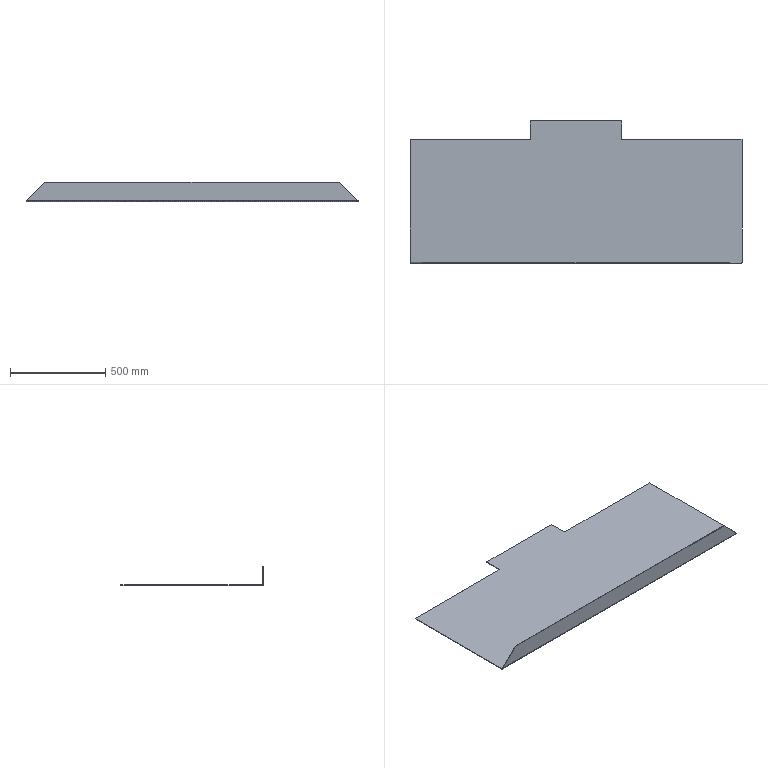Part | STEP file | Double-tube base plate SGN-1-02 | 1 solid | 18 faces | box 1740 x 745 x 100 mm | volume 3993617 mm3 | plane 14 | spline 2 | cylinder 2 | commonest cylinder face diameters 3 x1 9 x1